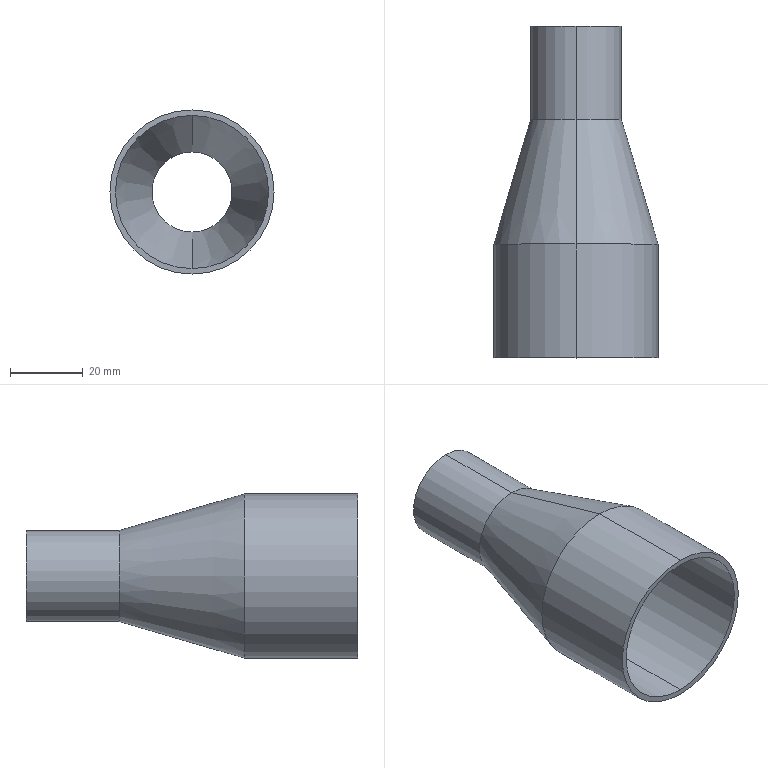Part | SolidWorks | features Revolution 1 | 1 solid | 14 faces | box 45 x 91 x 45 mm | volume 14846 mm3 | cylinder 8 | cone 4 | plane 2 | commonest cylinder face diameters 22 x2 25 x2 42 x2 45 x2
STEP:
#1=CARTESIAN_POINT('',(0.,19.9,12.5));
#2=VERTEX_POINT('',#1);
#3=CARTESIAN_POINT('',(0.,19.9,-12.5));
#4=VERTEX_POINT('',#3);
#5=CARTESIAN_POINT('',(0.,19.9,0.));
#6=DIRECTION('',(0.,1.,0.));
#7=DIRECTION('',(0.,0.,1.));
#8=AXIS2_PLACEMENT_3D('',#5,#6,#7);
#9=CIRCLE('',#8,12.5);
#10=EDGE_CURVE('',#2,#4,#9,.T.);
#11=ORIENTED_EDGE('',*,*,#10,.T.);
#12=CARTESIAN_POINT('',(0.,45.5,-12.5));
#13=VERTEX_POINT('',#12);
#14=CARTESIAN_POINT('',(0.,22.246,-12.5));
#15=DIRECTION('',(0.,1.,0.));
#16=VECTOR('',#15,1000.);
#17=LINE('',#14,#16);
#18=EDGE_CURVE('',#4,#13,#17,.T.);
#19=ORIENTED_EDGE('',*,*,#18,.T.);
#20=CARTESIAN_POINT('',(0.,45.5,12.5));
#21=VERTEX_POINT('',#20);
#22=CARTESIAN_POINT('',(0.,45.5,0.));
#23=DIRECTION('',(0.,1.,0.));
#24=DIRECTION('',(0.,0.,1.));
#25=AXIS2_PLACEMENT_3D('',#22,#23,#24);
#26=CIRCLE('',#25,12.5);
#27=EDGE_CURVE('',#21,#13,#26,.T.);
#28=ORIENTED_EDGE('',*,*,#27,.F.);
#29=CARTESIAN_POINT('',(0.,22.246,12.5));
#30=DIRECTION('',(0.,1.,0.));
#31=VECTOR('',#30,1000.);
#32=LINE('',#29,#31);
#33=EDGE_CURVE('',#2,#21,#32,.T.);
#34=ORIENTED_EDGE('',*,*,#33,.F.);
#35=EDGE_LOOP('',(#11,#19,#28,#34));
#36=FACE_OUTER_BOUND('',#35,.T.);
#37=CARTESIAN_POINT('',(0.,22.246,0.));
#38=DIRECTION('',(0.,1.,0.));
#39=DIRECTION('',(0.,0.,1.));
#40=AXIS2_PLACEMENT_3D('',#37,#38,#39);
#41=CYLINDRICAL_SURFACE('',#40,12.5);
#42=ADVANCED_FACE('',(#36),#41,.T.);
#43=ORIENTED_EDGE('',*,*,#10,.F.);
#44=CARTESIAN_POINT('',(0.,-14.3,22.5));
#45=VERTEX_POINT('',#44);
#46=CARTESIAN_POINT('',(0.,19.9,12.5));
#47=DIRECTION('',(0.,-0.9598,0.2806));
#48=VECTOR('',#47,1000.);
#49=LINE('',#46,#48);
#50=EDGE_CURVE('',#2,#45,#49,.T.);
#51=ORIENTED_EDGE('',*,*,#50,.T.);
#52=CARTESIAN_POINT('',(0.,-14.3,-22.5));
#53=VERTEX_POINT('',#52);
#54=CARTESIAN_POINT('',(0.,-14.3,0.));
#55=DIRECTION('',(0.,1.,0.));
#56=DIRECTION('',(0.,0.,1.));
#57=AXIS2_PLACEMENT_3D('',#54,#55,#56);
#58=CIRCLE('',#57,22.5);
#59=EDGE_CURVE('',#45,#53,#58,.T.);
#60=ORIENTED_EDGE('',*,*,#59,.T.);
#61=CARTESIAN_POINT('',(0.,19.9,-12.5));
#62=DIRECTION('',(0.,-0.9598,-0.2806));
#63=VECTOR('',#62,1000.);
#64=LINE('',#61,#63);
#65=EDGE_CURVE('',#4,#53,#64,.T.);
#66=ORIENTED_EDGE('',*,*,#65,.F.);
#67=EDGE_LOOP('',(#43,#51,#60,#66));
#68=FACE_OUTER_BOUND('',#67,.T.);
#69=CARTESIAN_POINT('',(0.,19.9,0.));
#70=DIRECTION('',(0.,-1.,0.));
#71=DIRECTION('',(0.,0.,-1.));
#72=AXIS2_PLACEMENT_3D('',#69,#70,#71);
#73=CONICAL_SURFACE('',#72,12.5,0.2845);
#74=ADVANCED_FACE('',(#68),#73,.T.);
#75=CARTESIAN_POINT('',(0.,-45.5,22.5));
#76=VERTEX_POINT('',#75);
#77=CARTESIAN_POINT('',(0.,-45.5,-22.5));
#78=VERTEX_POINT('',#77);
#79=CARTESIAN_POINT('',(0.,-45.5,0.));
#80=DIRECTION('',(0.,1.,0.));
#81=DIRECTION('',(0.,0.,1.));
#82=AXIS2_PLACEMENT_3D('',#79,#80,#81);
#83=CIRCLE('',#82,22.5);
#84=EDGE_CURVE('',#76,#78,#83,.T.);
#85=ORIENTED_EDGE('',*,*,#84,.T.);
#86=CARTESIAN_POINT('',(0.,22.246,-22.5));
#87=DIRECTION('',(0.,1.,0.));
#88=VECTOR('',#87,1000.);
#89=LINE('',#86,#88);
#90=EDGE_CURVE('',#78,#53,#89,.T.);
#91=ORIENTED_EDGE('',*,*,#90,.T.);
#92=ORIENTED_EDGE('',*,*,#59,.F.);
#93=CARTESIAN_POINT('',(0.,22.246,22.5));
#94=DIRECTION('',(0.,1.,0.));
#95=VECTOR('',#94,1000.);
#96=LINE('',#93,#95);
#97=EDGE_CURVE('',#76,#45,#96,.T.);
#98=ORIENTED_EDGE('',*,*,#97,.F.);
#99=EDGE_LOOP('',(#85,#91,#92,#98));
#100=FACE_OUTER_BOUND('',#99,.T.);
#101=CARTESIAN_POINT('',(0.,22.246,0.));
#102=DIRECTION('',(0.,1.,0.));
#103=DIRECTION('',(0.,0.,1.));
#104=AXIS2_PLACEMENT_3D('',#101,#102,#103);
#105=CYLINDRICAL_SURFACE('',#104,22.5);
#106=ADVANCED_FACE('',(#100),#105,.T.);
#107=CARTESIAN_POINT('',(0.,-45.5,-21.));
#108=VERTEX_POINT('',#107);
#109=CARTESIAN_POINT('',(0.,-45.5,21.));
#110=VERTEX_POINT('',#109);
#111=CARTESIAN_POINT('',(0.,-45.5,0.));
#112=DIRECTION('',(0.,1.,0.));
#113=DIRECTION('',(0.,0.,1.));
#114=AXIS2_PLACEMENT_3D('',#111,#112,#113);
#115=CIRCLE('',#114,21.);
#116=EDGE_CURVE('',#108,#110,#115,.T.);
#117=ORIENTED_EDGE('',*,*,#116,.F.);
#118=CARTESIAN_POINT('',(0.,-14.515,-21.));
#119=VERTEX_POINT('',#118);
#120=CARTESIAN_POINT('',(0.,22.246,-21.));
#121=DIRECTION('',(0.,1.,0.));
#122=VECTOR('',#121,1000.);
#123=LINE('',#120,#122);
#124=EDGE_CURVE('',#108,#119,#123,.T.);
#125=ORIENTED_EDGE('',*,*,#124,.T.);
#126=CARTESIAN_POINT('',(0.,-14.515,21.));
#127=VERTEX_POINT('',#126);
#128=CARTESIAN_POINT('',(0.,-14.515,0.));
#129=DIRECTION('',(0.,1.,0.));
#130=DIRECTION('',(0.,0.,1.));
#131=AXIS2_PLACEMENT_3D('',#128,#129,#130);
#132=CIRCLE('',#131,21.);
#133=EDGE_CURVE('',#119,#127,#132,.T.);
#134=ORIENTED_EDGE('',*,*,#133,.T.);
#135=CARTESIAN_POINT('',(0.,22.246,21.));
#136=DIRECTION('',(0.,1.,0.));
#137=VECTOR('',#136,1000.);
#138=LINE('',#135,#137);
#139=EDGE_CURVE('',#110,#127,#138,.T.);
#140=ORIENTED_EDGE('',*,*,#139,.F.);
#141=EDGE_LOOP('',(#117,#125,#134,#140));
#142=FACE_OUTER_BOUND('',#141,.T.);
#143=CARTESIAN_POINT('',(0.,22.246,0.));
#144=DIRECTION('',(0.,1.,0.));
#145=DIRECTION('',(0.,0.,1.));
#146=AXIS2_PLACEMENT_3D('',#143,#144,#145);
#147=CYLINDRICAL_SURFACE('',#146,21.);
#148=ADVANCED_FACE('',(#142),#147,.F.);
#149=CARTESIAN_POINT('',(0.,19.685,-11.));
#150=VERTEX_POINT('',#149);
#151=CARTESIAN_POINT('',(0.,19.685,11.));
#152=VERTEX_POINT('',#151);
#153=CARTESIAN_POINT('',(0.,19.685,0.));
#154=DIRECTION('',(0.,1.,0.));
#155=DIRECTION('',(0.,0.,1.));
#156=AXIS2_PLACEMENT_3D('',#153,#154,#155);
#157=CIRCLE('',#156,11.);
#158=EDGE_CURVE('',#150,#152,#157,.T.);
#159=ORIENTED_EDGE('',*,*,#158,.T.);
#160=CARTESIAN_POINT('',(0.,-14.515,21.));
#161=DIRECTION('',(0.,-0.9598,0.2806));
#162=VECTOR('',#161,1000.);
#163=LINE('',#160,#162);
#164=EDGE_CURVE('',#152,#127,#163,.T.);
#165=ORIENTED_EDGE('',*,*,#164,.T.);
#166=ORIENTED_EDGE('',*,*,#133,.F.);
#167=CARTESIAN_POINT('',(0.,-14.515,-21.));
#168=DIRECTION('',(0.,-0.9598,-0.2806));
#169=VECTOR('',#168,1000.);
#170=LINE('',#167,#169);
#171=EDGE_CURVE('',#150,#119,#170,.T.);
#172=ORIENTED_EDGE('',*,*,#171,.F.);
#173=EDGE_LOOP('',(#159,#165,#166,#172));
#174=FACE_OUTER_BOUND('',#173,.T.);
#175=CARTESIAN_POINT('',(0.,-14.515,0.));
#176=DIRECTION('',(0.,-1.,0.));
#177=DIRECTION('',(0.,0.,-1.));
#178=AXIS2_PLACEMENT_3D('',#175,#176,#177);
#179=CONICAL_SURFACE('',#178,21.,0.2845);
#180=ADVANCED_FACE('',(#174),#179,.F.);
#181=ORIENTED_EDGE('',*,*,#158,.F.);
#182=CARTESIAN_POINT('',(0.,45.5,-11.));
#183=VERTEX_POINT('',#182);
#184=CARTESIAN_POINT('',(0.,22.246,-11.));
#185=DIRECTION('',(0.,1.,0.));
#186=VECTOR('',#185,1000.);
#187=LINE('',#184,#186);
#188=EDGE_CURVE('',#150,#183,#187,.T.);
#189=ORIENTED_EDGE('',*,*,#188,.T.);
#190=CARTESIAN_POINT('',(0.,45.5,11.));
#191=VERTEX_POINT('',#190);
#192=CARTESIAN_POINT('',(0.,45.5,0.));
#193=DIRECTION('',(0.,1.,0.));
#194=DIRECTION('',(0.,0.,1.));
#195=AXIS2_PLACEMENT_3D('',#192,#193,#194);
#196=CIRCLE('',#195,11.);
#197=EDGE_CURVE('',#183,#191,#196,.T.);
#198=ORIENTED_EDGE('',*,*,#197,.T.);
#199=CARTESIAN_POINT('',(0.,22.246,11.));
#200=DIRECTION('',(0.,1.,0.));
#201=VECTOR('',#200,1000.);
#202=LINE('',#199,#201);
#203=EDGE_CURVE('',#152,#191,#202,.T.);
#204=ORIENTED_EDGE('',*,*,#203,.F.);
#205=EDGE_LOOP('',(#181,#189,#198,#204));
#206=FACE_OUTER_BOUND('',#205,.T.);
#207=CARTESIAN_POINT('',(0.,22.246,0.));
#208=DIRECTION('',(0.,1.,0.));
#209=DIRECTION('',(0.,0.,1.));
#210=AXIS2_PLACEMENT_3D('',#207,#208,#209);
#211=CYLINDRICAL_SURFACE('',#210,11.);
#212=ADVANCED_FACE('',(#206),#211,.F.);
#213=ORIENTED_EDGE('',*,*,#27,.T.);
#214=CARTESIAN_POINT('',(0.,45.5,0.));
#215=DIRECTION('',(0.,1.,0.));
#216=DIRECTION('',(0.,0.,1.));
#217=AXIS2_PLACEMENT_3D('',#214,#215,#216);
#218=CIRCLE('',#217,12.5);
#219=EDGE_CURVE('',#13,#21,#218,.T.);
#220=ORIENTED_EDGE('',*,*,#219,.T.);
#221=EDGE_LOOP('',(#213,#220));
#222=FACE_OUTER_BOUND('',#221,.T.);
#223=CARTESIAN_POINT('',(0.,45.5,0.));
#224=DIRECTION('',(0.,1.,0.));
#225=DIRECTION('',(0.,0.,1.));
#226=AXIS2_PLACEMENT_3D('',#223,#224,#225);
#227=CIRCLE('',#226,11.);
#228=EDGE_CURVE('',#191,#183,#227,.T.);
#229=ORIENTED_EDGE('',*,*,#228,.F.);
#230=ORIENTED_EDGE('',*,*,#197,.F.);
#231=EDGE_LOOP('',(#229,#230));
#232=FACE_BOUND('',#231,.T.);
#233=CARTESIAN_POINT('',(-12.5,45.5,0.));
#234=DIRECTION('',(0.,1.,0.));
#235=DIRECTION('',(0.,0.,1.));
#236=AXIS2_PLACEMENT_3D('',#233,#234,#235);
#237=PLANE('',#236);
#238=ADVANCED_FACE('',(#222,#232),#237,.T.);
#239=ORIENTED_EDGE('',*,*,#188,.F.);
#240=CARTESIAN_POINT('',(0.,19.685,0.));
#241=DIRECTION('',(0.,1.,0.));
#242=DIRECTION('',(0.,0.,1.));
#243=AXIS2_PLACEMENT_3D('',#240,#241,#242);
#244=CIRCLE('',#243,11.);
#245=EDGE_CURVE('',#152,#150,#244,.T.);
#246=ORIENTED_EDGE('',*,*,#245,.F.);
#247=ORIENTED_EDGE('',*,*,#203,.T.);
#248=ORIENTED_EDGE('',*,*,#228,.T.);
#249=EDGE_LOOP('',(#239,#246,#247,#248));
#250=FACE_OUTER_BOUND('',#249,.T.);
#251=CARTESIAN_POINT('',(0.,22.246,0.));
#252=DIRECTION('',(0.,1.,0.));
#253=DIRECTION('',(0.,0.,1.));
#254=AXIS2_PLACEMENT_3D('',#251,#252,#253);
#255=CYLINDRICAL_SURFACE('',#254,11.);
#256=ADVANCED_FACE('',(#250),#255,.F.);
#257=ORIENTED_EDGE('',*,*,#164,.F.);
#258=ORIENTED_EDGE('',*,*,#245,.T.);
#259=ORIENTED_EDGE('',*,*,#171,.T.);
#260=CARTESIAN_POINT('',(0.,-14.515,0.));
#261=DIRECTION('',(0.,1.,0.));
#262=DIRECTION('',(0.,0.,1.));
#263=AXIS2_PLACEMENT_3D('',#260,#261,#262);
#264=CIRCLE('',#263,21.);
#265=EDGE_CURVE('',#127,#119,#264,.T.);
#266=ORIENTED_EDGE('',*,*,#265,.F.);
#267=EDGE_LOOP('',(#257,#258,#259,#266));
#268=FACE_OUTER_BOUND('',#267,.T.);
#269=CARTESIAN_POINT('',(0.,-14.515,0.));
#270=DIRECTION('',(0.,-1.,0.));
#271=DIRECTION('',(0.,0.,-1.));
#272=AXIS2_PLACEMENT_3D('',#269,#270,#271);
#273=CONICAL_SURFACE('',#272,21.,0.2845);
#274=ADVANCED_FACE('',(#268),#273,.F.);
#275=ORIENTED_EDGE('',*,*,#124,.F.);
#276=CARTESIAN_POINT('',(0.,-45.5,0.));
#277=DIRECTION('',(0.,1.,0.));
#278=DIRECTION('',(0.,0.,1.));
#279=AXIS2_PLACEMENT_3D('',#276,#277,#278);
#280=CIRCLE('',#279,21.);
#281=EDGE_CURVE('',#110,#108,#280,.T.);
#282=ORIENTED_EDGE('',*,*,#281,.F.);
#283=ORIENTED_EDGE('',*,*,#139,.T.);
#284=ORIENTED_EDGE('',*,*,#265,.T.);
#285=EDGE_LOOP('',(#275,#282,#283,#284));
#286=FACE_OUTER_BOUND('',#285,.T.);
#287=CARTESIAN_POINT('',(0.,22.246,0.));
#288=DIRECTION('',(0.,1.,0.));
#289=DIRECTION('',(0.,0.,1.));
#290=AXIS2_PLACEMENT_3D('',#287,#288,#289);
#291=CYLINDRICAL_SURFACE('',#290,21.);
#292=ADVANCED_FACE('',(#286),#291,.F.);
#293=ORIENTED_EDGE('',*,*,#281,.T.);
#294=ORIENTED_EDGE('',*,*,#116,.T.);
#295=EDGE_LOOP('',(#293,#294));
#296=FACE_BOUND('',#295,.T.);
#297=ORIENTED_EDGE('',*,*,#84,.F.);
#298=CARTESIAN_POINT('',(0.,-45.5,0.));
#299=DIRECTION('',(0.,1.,0.));
#300=DIRECTION('',(0.,0.,1.));
#301=AXIS2_PLACEMENT_3D('',#298,#299,#300);
#302=CIRCLE('',#301,22.5);
#303=EDGE_CURVE('',#78,#76,#302,.T.);
#304=ORIENTED_EDGE('',*,*,#303,.F.);
#305=EDGE_LOOP('',(#297,#304));
#306=FACE_OUTER_BOUND('',#305,.T.);
#307=CARTESIAN_POINT('',(-22.5,-45.5,0.));
#308=DIRECTION('',(0.,-1.,0.));
#309=DIRECTION('',(0.,0.,-1.));
#310=AXIS2_PLACEMENT_3D('',#307,#308,#309);
#311=PLANE('',#310);
#312=ADVANCED_FACE('',(#296,#306),#311,.T.);
#313=ORIENTED_EDGE('',*,*,#90,.F.);
#314=ORIENTED_EDGE('',*,*,#303,.T.);
#315=ORIENTED_EDGE('',*,*,#97,.T.);
#316=CARTESIAN_POINT('',(0.,-14.3,0.));
#317=DIRECTION('',(0.,1.,0.));
#318=DIRECTION('',(0.,0.,1.));
#319=AXIS2_PLACEMENT_3D('',#316,#317,#318);
#320=CIRCLE('',#319,22.5);
#321=EDGE_CURVE('',#53,#45,#320,.T.);
#322=ORIENTED_EDGE('',*,*,#321,.F.);
#323=EDGE_LOOP('',(#313,#314,#315,#322));
#324=FACE_OUTER_BOUND('',#323,.T.);
#325=CARTESIAN_POINT('',(0.,22.246,0.));
#326=DIRECTION('',(0.,1.,0.));
#327=DIRECTION('',(0.,0.,1.));
#328=AXIS2_PLACEMENT_3D('',#325,#326,#327);
#329=CYLINDRICAL_SURFACE('',#328,22.5);
#330=ADVANCED_FACE('',(#324),#329,.T.);
#331=ORIENTED_EDGE('',*,*,#50,.F.);
#332=CARTESIAN_POINT('',(0.,19.9,0.));
#333=DIRECTION('',(0.,1.,0.));
#334=DIRECTION('',(0.,0.,1.));
#335=AXIS2_PLACEMENT_3D('',#332,#333,#334);
#336=CIRCLE('',#335,12.5);
#337=EDGE_CURVE('',#4,#2,#336,.T.);
#338=ORIENTED_EDGE('',*,*,#337,.F.);
#339=ORIENTED_EDGE('',*,*,#65,.T.);
#340=ORIENTED_EDGE('',*,*,#321,.T.);
#341=EDGE_LOOP('',(#331,#338,#339,#340));
#342=FACE_OUTER_BOUND('',#341,.T.);
#343=CARTESIAN_POINT('',(0.,19.9,0.));
#344=DIRECTION('',(0.,-1.,0.));
#345=DIRECTION('',(0.,0.,-1.));
#346=AXIS2_PLACEMENT_3D('',#343,#344,#345);
#347=CONICAL_SURFACE('',#346,12.5,0.2845);
#348=ADVANCED_FACE('',(#342),#347,.T.);
#349=ORIENTED_EDGE('',*,*,#18,.F.);
#350=ORIENTED_EDGE('',*,*,#337,.T.);
#351=ORIENTED_EDGE('',*,*,#33,.T.);
#352=ORIENTED_EDGE('',*,*,#219,.F.);
#353=EDGE_LOOP('',(#349,#350,#351,#352));
#354=FACE_OUTER_BOUND('',#353,.T.);
#355=CARTESIAN_POINT('',(0.,22.246,0.));
#356=DIRECTION('',(0.,1.,0.));
#357=DIRECTION('',(0.,0.,1.));
#358=AXIS2_PLACEMENT_3D('',#355,#356,#357);
#359=CYLINDRICAL_SURFACE('',#358,12.5);
#360=ADVANCED_FACE('',(#354),#359,.T.);
#361=CLOSED_SHELL('',(#42,#74,#106,#148,#180,#212,#238,#256,#274,#292,#312,#330,#348,#360));
#362=MANIFOLD_SOLID_BREP('',#361);
#363=CARTESIAN_POINT('',(0.,0.,0.));
#364=DIRECTION('',(0.,0.,1.));
#365=DIRECTION('',(1.,0.,0.));
#366=AXIS2_PLACEMENT_3D('',#363,#364,#365);
#367=(LENGTH_UNIT()NAMED_UNIT(*)SI_UNIT(.MILLI.,.METRE.));
#368=UNCERTAINTY_MEASURE_WITH_UNIT(LENGTH_MEASURE(0.00001),#367,'','');
#369=(NAMED_UNIT(*)PLANE_ANGLE_UNIT()SI_UNIT($,.RADIAN.));
#370=(NAMED_UNIT(*)SI_UNIT($,.STERADIAN.)SOLID_ANGLE_UNIT());
#371=(GEOMETRIC_REPRESENTATION_CONTEXT(3)GLOBAL_UNCERTAINTY_ASSIGNED_CONTEXT((#368))GLOBAL_UNIT_ASSIGNED_CONTEXT((#367,#369,#370))REPRESENTATION_CONTEXT('',''));
#372=ADVANCED_BREP_SHAPE_REPRESENTATION('',(#362,#366),#371);